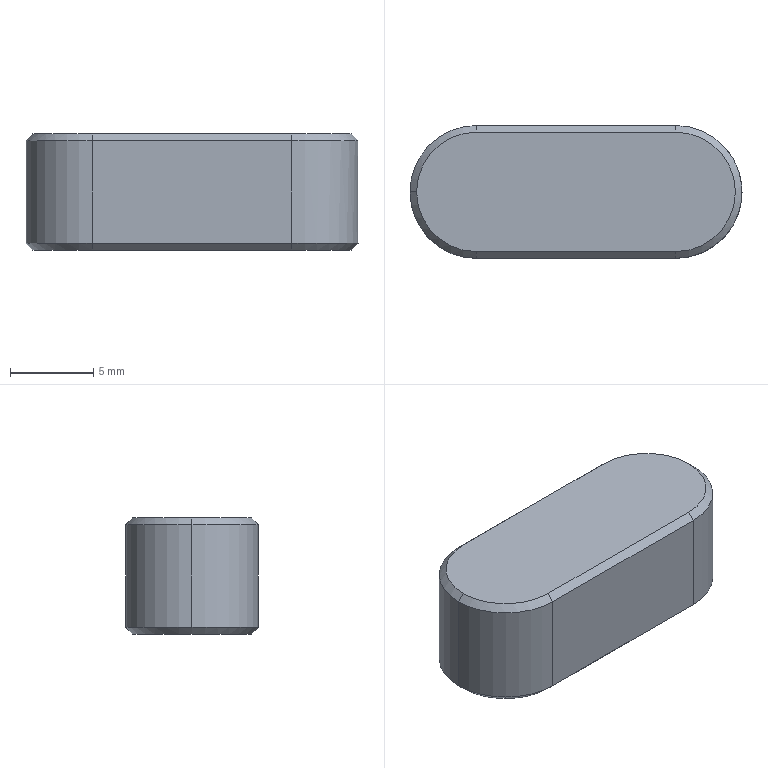Part | SolidWorks | features Boss 2, Chamfer 1, Extrusion 1 | 1 solid | 17 faces | box 20 x 8 x 7 mm | volume 1016 mm3 | plane 8 | cone 6 | cylinder 3 | commonest cylinder face diameters 8 x3
STEP:
#1=CARTESIAN_POINT('',(-15.6,0.,3.5));
#2=VERTEX_POINT('',#1);
#3=CARTESIAN_POINT('',(-12.,-3.6,3.5));
#4=VERTEX_POINT('',#3);
#5=CARTESIAN_POINT('',(-12.,0.,3.5));
#6=DIRECTION('',(0.,0.,1.));
#7=DIRECTION('',(-1.,0.,0.));
#8=AXIS2_PLACEMENT_3D('',#5,#6,#7);
#9=CIRCLE('',#8,3.6);
#10=EDGE_CURVE('',#2,#4,#9,.T.);
#11=ORIENTED_EDGE('',*,*,#10,.F.);
#12=CARTESIAN_POINT('',(-16.,0.,3.1));
#13=VERTEX_POINT('',#12);
#14=CARTESIAN_POINT('',(-15.6,0.,3.5));
#15=DIRECTION('',(-0.7071,0.,-0.7071));
#16=VECTOR('',#15,1000.);
#17=LINE('',#14,#16);
#18=EDGE_CURVE('',#2,#13,#17,.T.);
#19=ORIENTED_EDGE('',*,*,#18,.T.);
#20=CARTESIAN_POINT('',(-12.,-4.,3.1));
#21=VERTEX_POINT('',#20);
#22=CARTESIAN_POINT('',(-12.,0.,3.1));
#23=DIRECTION('',(0.,0.,-1.));
#24=DIRECTION('',(-1.,0.,0.));
#25=AXIS2_PLACEMENT_3D('',#22,#23,#24);
#26=CIRCLE('',#25,4.);
#27=EDGE_CURVE('',#21,#13,#26,.T.);
#28=ORIENTED_EDGE('',*,*,#27,.F.);
#29=CARTESIAN_POINT('',(-12.,-3.6,3.5));
#30=DIRECTION('',(0.,-0.7071,-0.7071));
#31=VECTOR('',#30,1000.);
#32=LINE('',#29,#31);
#33=EDGE_CURVE('',#4,#21,#32,.T.);
#34=ORIENTED_EDGE('',*,*,#33,.F.);
#35=EDGE_LOOP('',(#11,#19,#28,#34));
#36=FACE_OUTER_BOUND('',#35,.T.);
#37=CARTESIAN_POINT('',(-12.,0.,3.5));
#38=DIRECTION('',(0.,0.,-1.));
#39=DIRECTION('',(-1.,0.,0.));
#40=AXIS2_PLACEMENT_3D('',#37,#38,#39);
#41=CONICAL_SURFACE('',#40,3.6,0.7854);
#42=ADVANCED_FACE('',(#36),#41,.T.);
#43=CARTESIAN_POINT('',(3.6,0.,-3.5));
#44=VERTEX_POINT('',#43);
#45=CARTESIAN_POINT('',(0.,-3.6,-3.5));
#46=VERTEX_POINT('',#45);
#47=CARTESIAN_POINT('',(0.,0.,-3.5));
#48=DIRECTION('',(0.,0.,-1.));
#49=DIRECTION('',(-1.,0.,0.));
#50=AXIS2_PLACEMENT_3D('',#47,#48,#49);
#51=CIRCLE('',#50,3.6);
#52=EDGE_CURVE('',#44,#46,#51,.T.);
#53=ORIENTED_EDGE('',*,*,#52,.F.);
#54=CARTESIAN_POINT('',(4.,0.,-3.1));
#55=VERTEX_POINT('',#54);
#56=CARTESIAN_POINT('',(4.,0.,-3.1));
#57=DIRECTION('',(0.7071,0.,0.7071));
#58=VECTOR('',#57,1000.);
#59=LINE('',#56,#58);
#60=EDGE_CURVE('',#44,#55,#59,.T.);
#61=ORIENTED_EDGE('',*,*,#60,.T.);
#62=CARTESIAN_POINT('',(0.,-4.,-3.1));
#63=VERTEX_POINT('',#62);
#64=CARTESIAN_POINT('',(0.,0.,-3.1));
#65=DIRECTION('',(0.,0.,1.));
#66=DIRECTION('',(-1.,0.,0.));
#67=AXIS2_PLACEMENT_3D('',#64,#65,#66);
#68=CIRCLE('',#67,4.);
#69=EDGE_CURVE('',#63,#55,#68,.T.);
#70=ORIENTED_EDGE('',*,*,#69,.F.);
#71=CARTESIAN_POINT('',(0.,-3.6,-3.5));
#72=DIRECTION('',(0.,-0.7071,0.7071));
#73=VECTOR('',#72,1000.);
#74=LINE('',#71,#73);
#75=EDGE_CURVE('',#46,#63,#74,.T.);
#76=ORIENTED_EDGE('',*,*,#75,.F.);
#77=EDGE_LOOP('',(#53,#61,#70,#76));
#78=FACE_OUTER_BOUND('',#77,.T.);
#79=CARTESIAN_POINT('',(0.,0.,-3.1));
#80=DIRECTION('',(0.,0.,1.));
#81=DIRECTION('',(1.,0.,0.));
#82=AXIS2_PLACEMENT_3D('',#79,#80,#81);
#83=CONICAL_SURFACE('',#82,4.,0.7854);
#84=ADVANCED_FACE('',(#78),#83,.T.);
#85=ORIENTED_EDGE('',*,*,#27,.T.);
#86=CARTESIAN_POINT('',(-16.,0.,-3.1));
#87=VERTEX_POINT('',#86);
#88=CARTESIAN_POINT('',(-16.,0.,3.5));
#89=DIRECTION('',(0.,0.,-1.));
#90=VECTOR('',#89,1000.);
#91=LINE('',#88,#90);
#92=EDGE_CURVE('',#13,#87,#91,.T.);
#93=ORIENTED_EDGE('',*,*,#92,.T.);
#94=CARTESIAN_POINT('',(-12.,-4.,-3.1));
#95=VERTEX_POINT('',#94);
#96=CARTESIAN_POINT('',(-12.,0.,-3.1));
#97=DIRECTION('',(0.,0.,1.));
#98=DIRECTION('',(-1.,0.,0.));
#99=AXIS2_PLACEMENT_3D('',#96,#97,#98);
#100=CIRCLE('',#99,4.);
#101=EDGE_CURVE('',#87,#95,#100,.T.);
#102=ORIENTED_EDGE('',*,*,#101,.T.);
#103=CARTESIAN_POINT('',(-12.,-4.,3.5));
#104=DIRECTION('',(0.,0.,-1.));
#105=VECTOR('',#104,1000.);
#106=LINE('',#103,#105);
#107=EDGE_CURVE('',#21,#95,#106,.T.);
#108=ORIENTED_EDGE('',*,*,#107,.F.);
#109=EDGE_LOOP('',(#85,#93,#102,#108));
#110=FACE_OUTER_BOUND('',#109,.T.);
#111=CARTESIAN_POINT('',(-12.,0.,3.5));
#112=DIRECTION('',(0.,0.,-1.));
#113=DIRECTION('',(-1.,0.,0.));
#114=AXIS2_PLACEMENT_3D('',#111,#112,#113);
#115=CYLINDRICAL_SURFACE('',#114,4.);
#116=ADVANCED_FACE('',(#110),#115,.T.);
#117=ORIENTED_EDGE('',*,*,#92,.F.);
#118=CARTESIAN_POINT('',(-12.,4.,3.1));
#119=VERTEX_POINT('',#118);
#120=CARTESIAN_POINT('',(-12.,0.,3.1));
#121=DIRECTION('',(0.,0.,-1.));
#122=DIRECTION('',(-1.,0.,0.));
#123=AXIS2_PLACEMENT_3D('',#120,#121,#122);
#124=CIRCLE('',#123,4.);
#125=EDGE_CURVE('',#13,#119,#124,.T.);
#126=ORIENTED_EDGE('',*,*,#125,.T.);
#127=CARTESIAN_POINT('',(-12.,4.,-3.1));
#128=VERTEX_POINT('',#127);
#129=CARTESIAN_POINT('',(-12.,4.,3.5));
#130=DIRECTION('',(0.,0.,-1.));
#131=VECTOR('',#130,1000.);
#132=LINE('',#129,#131);
#133=EDGE_CURVE('',#119,#128,#132,.T.);
#134=ORIENTED_EDGE('',*,*,#133,.T.);
#135=CARTESIAN_POINT('',(-12.,0.,-3.1));
#136=DIRECTION('',(0.,0.,1.));
#137=DIRECTION('',(-1.,0.,0.));
#138=AXIS2_PLACEMENT_3D('',#135,#136,#137);
#139=CIRCLE('',#138,4.);
#140=EDGE_CURVE('',#128,#87,#139,.T.);
#141=ORIENTED_EDGE('',*,*,#140,.T.);
#142=EDGE_LOOP('',(#117,#126,#134,#141));
#143=FACE_OUTER_BOUND('',#142,.T.);
#144=CARTESIAN_POINT('',(-12.,0.,3.5));
#145=DIRECTION('',(0.,0.,-1.));
#146=DIRECTION('',(-1.,0.,0.));
#147=AXIS2_PLACEMENT_3D('',#144,#145,#146);
#148=CYLINDRICAL_SURFACE('',#147,4.);
#149=ADVANCED_FACE('',(#143),#148,.T.);
#150=ORIENTED_EDGE('',*,*,#107,.T.);
#151=CARTESIAN_POINT('',(0.,-4.,-3.1));
#152=DIRECTION('',(1.,0.,0.));
#153=VECTOR('',#152,1000.);
#154=LINE('',#151,#153);
#155=EDGE_CURVE('',#95,#63,#154,.T.);
#156=ORIENTED_EDGE('',*,*,#155,.T.);
#157=CARTESIAN_POINT('',(0.,-4.,3.1));
#158=VERTEX_POINT('',#157);
#159=CARTESIAN_POINT('',(0.,-4.,3.5));
#160=DIRECTION('',(0.,0.,-1.));
#161=VECTOR('',#160,1000.);
#162=LINE('',#159,#161);
#163=EDGE_CURVE('',#158,#63,#162,.T.);
#164=ORIENTED_EDGE('',*,*,#163,.F.);
#165=CARTESIAN_POINT('',(0.,-4.,3.1));
#166=DIRECTION('',(-1.,0.,0.));
#167=VECTOR('',#166,1000.);
#168=LINE('',#165,#167);
#169=EDGE_CURVE('',#158,#21,#168,.T.);
#170=ORIENTED_EDGE('',*,*,#169,.T.);
#171=EDGE_LOOP('',(#150,#156,#164,#170));
#172=FACE_OUTER_BOUND('',#171,.T.);
#173=CARTESIAN_POINT('',(0.,-4.,3.5));
#174=DIRECTION('',(0.,1.,0.));
#175=DIRECTION('',(-1.,0.,0.));
#176=AXIS2_PLACEMENT_3D('',#173,#174,#175);
#177=PLANE('',#176);
#178=ADVANCED_FACE('',(#172),#177,.F.);
#179=CARTESIAN_POINT('',(0.,4.,3.1));
#180=VERTEX_POINT('',#179);
#181=CARTESIAN_POINT('',(0.,4.,-3.1));
#182=VERTEX_POINT('',#181);
#183=CARTESIAN_POINT('',(0.,4.,3.5));
#184=DIRECTION('',(0.,0.,-1.));
#185=VECTOR('',#184,1000.);
#186=LINE('',#183,#185);
#187=EDGE_CURVE('',#180,#182,#186,.T.);
#188=ORIENTED_EDGE('',*,*,#187,.F.);
#189=CARTESIAN_POINT('',(0.,0.,3.1));
#190=DIRECTION('',(0.,0.,-1.));
#191=DIRECTION('',(-1.,0.,0.));
#192=AXIS2_PLACEMENT_3D('',#189,#190,#191);
#193=CIRCLE('',#192,4.);
#194=EDGE_CURVE('',#180,#158,#193,.T.);
#195=ORIENTED_EDGE('',*,*,#194,.T.);
#196=ORIENTED_EDGE('',*,*,#163,.T.);
#197=ORIENTED_EDGE('',*,*,#69,.T.);
#198=CARTESIAN_POINT('',(0.,0.,-3.1));
#199=DIRECTION('',(0.,0.,1.));
#200=DIRECTION('',(-1.,0.,0.));
#201=AXIS2_PLACEMENT_3D('',#198,#199,#200);
#202=CIRCLE('',#201,4.);
#203=EDGE_CURVE('',#55,#182,#202,.T.);
#204=ORIENTED_EDGE('',*,*,#203,.T.);
#205=EDGE_LOOP('',(#188,#195,#196,#197,#204));
#206=FACE_OUTER_BOUND('',#205,.T.);
#207=CARTESIAN_POINT('',(0.,0.,3.5));
#208=DIRECTION('',(0.,0.,-1.));
#209=DIRECTION('',(-1.,0.,0.));
#210=AXIS2_PLACEMENT_3D('',#207,#208,#209);
#211=CYLINDRICAL_SURFACE('',#210,4.);
#212=ADVANCED_FACE('',(#206),#211,.T.);
#213=ORIENTED_EDGE('',*,*,#133,.F.);
#214=CARTESIAN_POINT('',(-12.,4.,3.1));
#215=DIRECTION('',(1.,0.,0.));
#216=VECTOR('',#215,1000.);
#217=LINE('',#214,#216);
#218=EDGE_CURVE('',#119,#180,#217,.T.);
#219=ORIENTED_EDGE('',*,*,#218,.T.);
#220=ORIENTED_EDGE('',*,*,#187,.T.);
#221=CARTESIAN_POINT('',(-12.,4.,-3.1));
#222=DIRECTION('',(-1.,0.,0.));
#223=VECTOR('',#222,1000.);
#224=LINE('',#221,#223);
#225=EDGE_CURVE('',#182,#128,#224,.T.);
#226=ORIENTED_EDGE('',*,*,#225,.T.);
#227=EDGE_LOOP('',(#213,#219,#220,#226));
#228=FACE_OUTER_BOUND('',#227,.T.);
#229=CARTESIAN_POINT('',(-12.,4.,3.5));
#230=DIRECTION('',(0.,-1.,0.));
#231=DIRECTION('',(0.,0.,-1.));
#232=AXIS2_PLACEMENT_3D('',#229,#230,#231);
#233=PLANE('',#232);
#234=ADVANCED_FACE('',(#228),#233,.F.);
#235=CARTESIAN_POINT('',(-12.,3.6,3.5));
#236=VERTEX_POINT('',#235);
#237=CARTESIAN_POINT('',(-12.,0.,3.5));
#238=DIRECTION('',(0.,0.,1.));
#239=DIRECTION('',(-1.,0.,0.));
#240=AXIS2_PLACEMENT_3D('',#237,#238,#239);
#241=CIRCLE('',#240,3.6);
#242=EDGE_CURVE('',#236,#2,#241,.T.);
#243=ORIENTED_EDGE('',*,*,#242,.T.);
#244=ORIENTED_EDGE('',*,*,#10,.T.);
#245=CARTESIAN_POINT('',(0.,-3.6,3.5));
#246=VERTEX_POINT('',#245);
#247=CARTESIAN_POINT('',(-12.,-3.6,3.5));
#248=DIRECTION('',(1.,0.,0.));
#249=VECTOR('',#248,1000.);
#250=LINE('',#247,#249);
#251=EDGE_CURVE('',#4,#246,#250,.T.);
#252=ORIENTED_EDGE('',*,*,#251,.T.);
#253=CARTESIAN_POINT('',(0.,3.6,3.5));
#254=VERTEX_POINT('',#253);
#255=CARTESIAN_POINT('',(0.,0.,3.5));
#256=DIRECTION('',(0.,0.,1.));
#257=DIRECTION('',(-1.,0.,0.));
#258=AXIS2_PLACEMENT_3D('',#255,#256,#257);
#259=CIRCLE('',#258,3.6);
#260=EDGE_CURVE('',#246,#254,#259,.T.);
#261=ORIENTED_EDGE('',*,*,#260,.T.);
#262=CARTESIAN_POINT('',(-12.,3.6,3.5));
#263=DIRECTION('',(-1.,0.,0.));
#264=VECTOR('',#263,1000.);
#265=LINE('',#262,#264);
#266=EDGE_CURVE('',#254,#236,#265,.T.);
#267=ORIENTED_EDGE('',*,*,#266,.T.);
#268=EDGE_LOOP('',(#243,#244,#252,#261,#267));
#269=FACE_OUTER_BOUND('',#268,.T.);
#270=CARTESIAN_POINT('',(-12.,0.,3.5));
#271=DIRECTION('',(0.,0.,-1.));
#272=DIRECTION('',(-1.,0.,0.));
#273=AXIS2_PLACEMENT_3D('',#270,#271,#272);
#274=PLANE('',#273);
#275=ADVANCED_FACE('',(#269),#274,.F.);
#276=CARTESIAN_POINT('',(0.,3.6,-3.5));
#277=VERTEX_POINT('',#276);
#278=CARTESIAN_POINT('',(0.,0.,-3.5));
#279=DIRECTION('',(0.,0.,-1.));
#280=DIRECTION('',(-1.,0.,0.));
#281=AXIS2_PLACEMENT_3D('',#278,#279,#280);
#282=CIRCLE('',#281,3.6);
#283=EDGE_CURVE('',#277,#44,#282,.T.);
#284=ORIENTED_EDGE('',*,*,#283,.T.);
#285=ORIENTED_EDGE('',*,*,#52,.T.);
#286=CARTESIAN_POINT('',(-12.,-3.6,-3.5));
#287=VERTEX_POINT('',#286);
#288=CARTESIAN_POINT('',(-12.,-3.6,-3.5));
#289=DIRECTION('',(-1.,0.,0.));
#290=VECTOR('',#289,1000.);
#291=LINE('',#288,#290);
#292=EDGE_CURVE('',#46,#287,#291,.T.);
#293=ORIENTED_EDGE('',*,*,#292,.T.);
#294=CARTESIAN_POINT('',(-12.,3.6,-3.5));
#295=VERTEX_POINT('',#294);
#296=CARTESIAN_POINT('',(-12.,0.,-3.5));
#297=DIRECTION('',(0.,0.,-1.));
#298=DIRECTION('',(-1.,0.,0.));
#299=AXIS2_PLACEMENT_3D('',#296,#297,#298);
#300=CIRCLE('',#299,3.6);
#301=EDGE_CURVE('',#287,#295,#300,.T.);
#302=ORIENTED_EDGE('',*,*,#301,.T.);
#303=CARTESIAN_POINT('',(0.,3.6,-3.5));
#304=DIRECTION('',(1.,0.,0.));
#305=VECTOR('',#304,1000.);
#306=LINE('',#303,#305);
#307=EDGE_CURVE('',#295,#277,#306,.T.);
#308=ORIENTED_EDGE('',*,*,#307,.T.);
#309=EDGE_LOOP('',(#284,#285,#293,#302,#308));
#310=FACE_OUTER_BOUND('',#309,.T.);
#311=CARTESIAN_POINT('',(-12.,0.,-3.5));
#312=DIRECTION('',(0.,0.,-1.));
#313=DIRECTION('',(-1.,0.,0.));
#314=AXIS2_PLACEMENT_3D('',#311,#312,#313);
#315=PLANE('',#314);
#316=ADVANCED_FACE('',(#310),#315,.T.);
#317=CARTESIAN_POINT('',(0.,3.6,-3.5));
#318=DIRECTION('',(0.,0.7071,0.7071));
#319=VECTOR('',#318,1000.);
#320=LINE('',#317,#319);
#321=EDGE_CURVE('',#277,#182,#320,.T.);
#322=ORIENTED_EDGE('',*,*,#321,.F.);
#323=ORIENTED_EDGE('',*,*,#307,.F.);
#324=CARTESIAN_POINT('',(-12.,4.,-3.1));
#325=DIRECTION('',(0.,-0.7071,-0.7071));
#326=VECTOR('',#325,1000.);
#327=LINE('',#324,#326);
#328=EDGE_CURVE('',#128,#295,#327,.T.);
#329=ORIENTED_EDGE('',*,*,#328,.F.);
#330=ORIENTED_EDGE('',*,*,#225,.F.);
#331=EDGE_LOOP('',(#322,#323,#329,#330));
#332=FACE_OUTER_BOUND('',#331,.T.);
#333=CARTESIAN_POINT('',(-12.,4.,-3.1));
#334=DIRECTION('',(0.,0.7071,-0.7071));
#335=DIRECTION('',(0.,0.7071,0.7071));
#336=AXIS2_PLACEMENT_3D('',#333,#334,#335);
#337=PLANE('',#336);
#338=ADVANCED_FACE('',(#332),#337,.T.);
#339=ORIENTED_EDGE('',*,*,#328,.T.);
#340=ORIENTED_EDGE('',*,*,#301,.F.);
#341=CARTESIAN_POINT('',(-12.,-4.,-3.1));
#342=DIRECTION('',(0.,0.7071,-0.7071));
#343=VECTOR('',#342,1000.);
#344=LINE('',#341,#343);
#345=EDGE_CURVE('',#95,#287,#344,.T.);
#346=ORIENTED_EDGE('',*,*,#345,.F.);
#347=ORIENTED_EDGE('',*,*,#101,.F.);
#348=ORIENTED_EDGE('',*,*,#140,.F.);
#349=EDGE_LOOP('',(#339,#340,#346,#347,#348));
#350=FACE_OUTER_BOUND('',#349,.T.);
#351=CARTESIAN_POINT('',(-12.,0.,-3.1));
#352=DIRECTION('',(0.,0.,1.));
#353=DIRECTION('',(1.,0.,0.));
#354=AXIS2_PLACEMENT_3D('',#351,#352,#353);
#355=CONICAL_SURFACE('',#354,4.,0.7854);
#356=ADVANCED_FACE('',(#350),#355,.T.);
#357=ORIENTED_EDGE('',*,*,#60,.F.);
#358=ORIENTED_EDGE('',*,*,#283,.F.);
#359=ORIENTED_EDGE('',*,*,#321,.T.);
#360=ORIENTED_EDGE('',*,*,#203,.F.);
#361=EDGE_LOOP('',(#357,#358,#359,#360));
#362=FACE_OUTER_BOUND('',#361,.T.);
#363=CARTESIAN_POINT('',(0.,0.,-3.1));
#364=DIRECTION('',(0.,0.,1.));
#365=DIRECTION('',(1.,0.,0.));
#366=AXIS2_PLACEMENT_3D('',#363,#364,#365);
#367=CONICAL_SURFACE('',#366,4.,0.7854);
#368=ADVANCED_FACE('',(#362),#367,.T.);
#369=ORIENTED_EDGE('',*,*,#345,.T.);
#370=ORIENTED_EDGE('',*,*,#292,.F.);
#371=ORIENTED_EDGE('',*,*,#75,.T.);
#372=ORIENTED_EDGE('',*,*,#155,.F.);
#373=EDGE_LOOP('',(#369,#370,#371,#372));
#374=FACE_OUTER_BOUND('',#373,.T.);
#375=CARTESIAN_POINT('',(0.,-4.,-3.1));
#376=DIRECTION('',(0.,-0.7071,-0.7071));
#377=DIRECTION('',(0.,0.7071,-0.7071));
#378=AXIS2_PLACEMENT_3D('',#375,#376,#377);
#379=PLANE('',#378);
#380=ADVANCED_FACE('',(#374),#379,.T.);
#381=CARTESIAN_POINT('',(0.,4.,3.1));
#382=DIRECTION('',(0.,-0.7071,0.7071));
#383=VECTOR('',#382,1000.);
#384=LINE('',#381,#383);
#385=EDGE_CURVE('',#180,#254,#384,.T.);
#386=ORIENTED_EDGE('',*,*,#385,.F.);
#387=ORIENTED_EDGE('',*,*,#218,.F.);
#388=CARTESIAN_POINT('',(-12.,3.6,3.5));
#389=DIRECTION('',(0.,0.7071,-0.7071));
#390=VECTOR('',#389,1000.);
#391=LINE('',#388,#390);
#392=EDGE_CURVE('',#236,#119,#391,.T.);
#393=ORIENTED_EDGE('',*,*,#392,.F.);
#394=ORIENTED_EDGE('',*,*,#266,.F.);
#395=EDGE_LOOP('',(#386,#387,#393,#394));
#396=FACE_OUTER_BOUND('',#395,.T.);
#397=CARTESIAN_POINT('',(-12.,3.6,3.5));
#398=DIRECTION('',(0.,-0.7071,-0.7071));
#399=DIRECTION('',(0.,0.7071,-0.7071));
#400=AXIS2_PLACEMENT_3D('',#397,#398,#399);
#401=PLANE('',#400);
#402=ADVANCED_FACE('',(#396),#401,.F.);
#403=ORIENTED_EDGE('',*,*,#18,.F.);
#404=ORIENTED_EDGE('',*,*,#242,.F.);
#405=ORIENTED_EDGE('',*,*,#392,.T.);
#406=ORIENTED_EDGE('',*,*,#125,.F.);
#407=EDGE_LOOP('',(#403,#404,#405,#406));
#408=FACE_OUTER_BOUND('',#407,.T.);
#409=CARTESIAN_POINT('',(-12.,0.,3.5));
#410=DIRECTION('',(0.,0.,-1.));
#411=DIRECTION('',(-1.,0.,0.));
#412=AXIS2_PLACEMENT_3D('',#409,#410,#411);
#413=CONICAL_SURFACE('',#412,3.6,0.7854);
#414=ADVANCED_FACE('',(#408),#413,.T.);
#415=ORIENTED_EDGE('',*,*,#385,.T.);
#416=ORIENTED_EDGE('',*,*,#260,.F.);
#417=CARTESIAN_POINT('',(0.,-4.,3.1));
#418=DIRECTION('',(0.,0.7071,0.7071));
#419=VECTOR('',#418,1000.);
#420=LINE('',#417,#419);
#421=EDGE_CURVE('',#158,#246,#420,.T.);
#422=ORIENTED_EDGE('',*,*,#421,.F.);
#423=ORIENTED_EDGE('',*,*,#194,.F.);
#424=EDGE_LOOP('',(#415,#416,#422,#423));
#425=FACE_OUTER_BOUND('',#424,.T.);
#426=CARTESIAN_POINT('',(0.,0.,3.5));
#427=DIRECTION('',(0.,0.,-1.));
#428=DIRECTION('',(-1.,0.,0.));
#429=AXIS2_PLACEMENT_3D('',#426,#427,#428);
#430=CONICAL_SURFACE('',#429,3.6,0.7854);
#431=ADVANCED_FACE('',(#425),#430,.T.);
#432=ORIENTED_EDGE('',*,*,#33,.T.);
#433=ORIENTED_EDGE('',*,*,#169,.F.);
#434=ORIENTED_EDGE('',*,*,#421,.T.);
#435=ORIENTED_EDGE('',*,*,#251,.F.);
#436=EDGE_LOOP('',(#432,#433,#434,#435));
#437=FACE_OUTER_BOUND('',#436,.T.);
#438=CARTESIAN_POINT('',(-12.,-3.6,3.5));
#439=DIRECTION('',(0.,0.7071,-0.7071));
#440=DIRECTION('',(0.,0.7071,0.7071));
#441=AXIS2_PLACEMENT_3D('',#438,#439,#440);
#442=PLANE('',#441);
#443=ADVANCED_FACE('',(#437),#442,.F.);
#444=CLOSED_SHELL('',(#42,#84,#116,#149,#178,#212,#234,#275,#316,#338,#356,#368,#380,#402,#414,#431,#443));
#445=MANIFOLD_SOLID_BREP('',#444);
#446=CARTESIAN_POINT('',(0.,0.,0.));
#447=DIRECTION('',(0.,0.,1.));
#448=DIRECTION('',(1.,0.,0.));
#449=AXIS2_PLACEMENT_3D('',#446,#447,#448);
#450=(LENGTH_UNIT()NAMED_UNIT(*)SI_UNIT(.MILLI.,.METRE.));
#451=UNCERTAINTY_MEASURE_WITH_UNIT(LENGTH_MEASURE(0.00001),#450,'','');
#452=(NAMED_UNIT(*)PLANE_ANGLE_UNIT()SI_UNIT($,.RADIAN.));
#453=(NAMED_UNIT(*)SI_UNIT($,.STERADIAN.)SOLID_ANGLE_UNIT());
#454=(GEOMETRIC_REPRESENTATION_CONTEXT(3)GLOBAL_UNCERTAINTY_ASSIGNED_CONTEXT((#451))GLOBAL_UNIT_ASSIGNED_CONTEXT((#450,#452,#453))REPRESENTATION_CONTEXT('',''));
#455=ADVANCED_BREP_SHAPE_REPRESENTATION('',(#445,#449),#454);